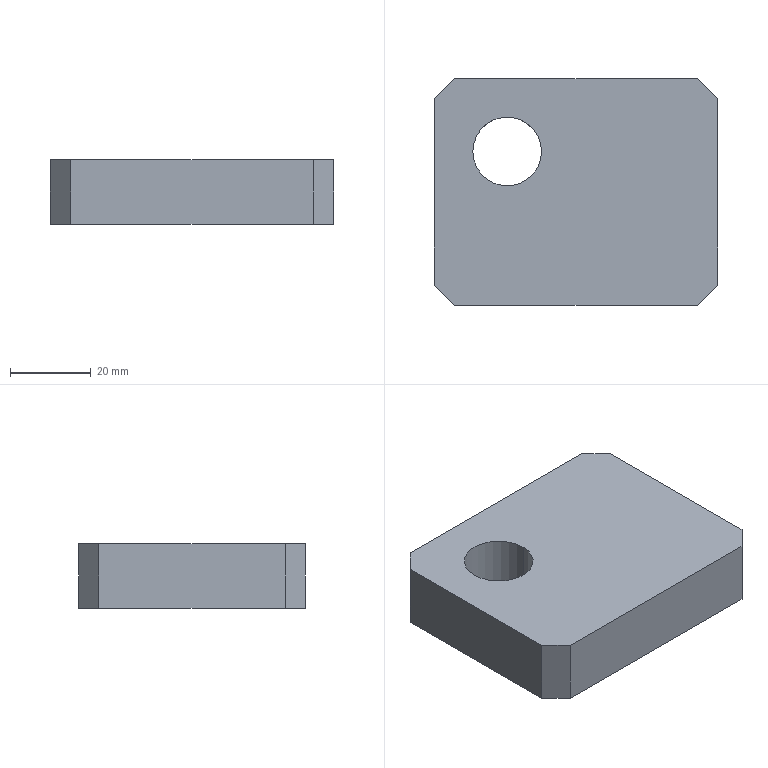Part | SolidWorks | features FlatPattern 1, SMBaseFlange 1, SheetMetal 1 | 1 solid | 12 faces | box 70 x 56 x 16 mm | volume 58288 mm3 | plane 10 | cylinder 2 | commonest cylinder face diameters 17 x2
STEP:
#1=CARTESIAN_POINT('',(9.5,-18.,-16.));
#2=VERTEX_POINT('',#1);
#3=CARTESIAN_POINT('',(26.5,-18.,-16.));
#4=VERTEX_POINT('',#3);
#5=CARTESIAN_POINT('',(18.,-18.,-16.));
#6=DIRECTION('',(0.,0.,1.));
#7=DIRECTION('',(1.,0.,0.));
#8=AXIS2_PLACEMENT_3D('',#5,#6,#7);
#9=CIRCLE('',#8,8.5);
#10=EDGE_CURVE('',#2,#4,#9,.T.);
#11=ORIENTED_EDGE('',*,*,#10,.F.);
#12=CARTESIAN_POINT('',(9.5,-18.,0.));
#13=VERTEX_POINT('',#12);
#14=CARTESIAN_POINT('',(9.5,-18.,-16.));
#15=DIRECTION('',(0.,0.,1.));
#16=VECTOR('',#15,1000.);
#17=LINE('',#14,#16);
#18=EDGE_CURVE('',#2,#13,#17,.T.);
#19=ORIENTED_EDGE('',*,*,#18,.T.);
#20=CARTESIAN_POINT('',(26.5,-18.,0.));
#21=VERTEX_POINT('',#20);
#22=CARTESIAN_POINT('',(18.,-18.,0.));
#23=DIRECTION('',(0.,0.,1.));
#24=DIRECTION('',(1.,0.,0.));
#25=AXIS2_PLACEMENT_3D('',#22,#23,#24);
#26=CIRCLE('',#25,8.5);
#27=EDGE_CURVE('',#13,#21,#26,.T.);
#28=ORIENTED_EDGE('',*,*,#27,.T.);
#29=CARTESIAN_POINT('',(26.5,-18.,-16.));
#30=DIRECTION('',(0.,0.,1.));
#31=VECTOR('',#30,1000.);
#32=LINE('',#29,#31);
#33=EDGE_CURVE('',#4,#21,#32,.T.);
#34=ORIENTED_EDGE('',*,*,#33,.F.);
#35=EDGE_LOOP('',(#11,#19,#28,#34));
#36=FACE_OUTER_BOUND('',#35,.T.);
#37=CARTESIAN_POINT('',(18.,-18.,-16.));
#38=DIRECTION('',(0.,0.,1.));
#39=DIRECTION('',(1.,0.,0.));
#40=AXIS2_PLACEMENT_3D('',#37,#38,#39);
#41=CYLINDRICAL_SURFACE('',#40,8.5);
#42=ADVANCED_FACE('',(#36),#41,.F.);
#43=CARTESIAN_POINT('',(65.,0.,0.));
#44=VERTEX_POINT('',#43);
#45=CARTESIAN_POINT('',(5.,0.,0.));
#46=VERTEX_POINT('',#45);
#47=CARTESIAN_POINT('',(5.,0.,0.));
#48=DIRECTION('',(-1.,0.,0.));
#49=VECTOR('',#48,1000.);
#50=LINE('',#47,#49);
#51=EDGE_CURVE('',#44,#46,#50,.T.);
#52=ORIENTED_EDGE('',*,*,#51,.F.);
#53=CARTESIAN_POINT('',(65.,0.,-16.));
#54=VERTEX_POINT('',#53);
#55=CARTESIAN_POINT('',(65.,0.,-16.));
#56=DIRECTION('',(0.,0.,1.));
#57=VECTOR('',#56,1000.);
#58=LINE('',#55,#57);
#59=EDGE_CURVE('',#54,#44,#58,.T.);
#60=ORIENTED_EDGE('',*,*,#59,.F.);
#61=CARTESIAN_POINT('',(5.,0.,-16.));
#62=VERTEX_POINT('',#61);
#63=CARTESIAN_POINT('',(5.,0.,-16.));
#64=DIRECTION('',(-1.,0.,0.));
#65=VECTOR('',#64,1000.);
#66=LINE('',#63,#65);
#67=EDGE_CURVE('',#54,#62,#66,.T.);
#68=ORIENTED_EDGE('',*,*,#67,.T.);
#69=CARTESIAN_POINT('',(5.,0.,-16.));
#70=DIRECTION('',(0.,0.,1.));
#71=VECTOR('',#70,1000.);
#72=LINE('',#69,#71);
#73=EDGE_CURVE('',#62,#46,#72,.T.);
#74=ORIENTED_EDGE('',*,*,#73,.T.);
#75=EDGE_LOOP('',(#52,#60,#68,#74));
#76=FACE_OUTER_BOUND('',#75,.T.);
#77=CARTESIAN_POINT('',(5.,0.,-16.));
#78=DIRECTION('',(0.,1.,0.));
#79=DIRECTION('',(0.,0.,1.));
#80=AXIS2_PLACEMENT_3D('',#77,#78,#79);
#81=PLANE('',#80);
#82=ADVANCED_FACE('',(#76),#81,.T.);
#83=CARTESIAN_POINT('',(70.,-5.,0.));
#84=VERTEX_POINT('',#83);
#85=CARTESIAN_POINT('',(65.,0.,0.));
#86=DIRECTION('',(-0.7071,0.7071,0.));
#87=VECTOR('',#86,1000.);
#88=LINE('',#85,#87);
#89=EDGE_CURVE('',#84,#44,#88,.T.);
#90=ORIENTED_EDGE('',*,*,#89,.F.);
#91=CARTESIAN_POINT('',(70.,-5.,-16.));
#92=VERTEX_POINT('',#91);
#93=CARTESIAN_POINT('',(70.,-5.,-16.));
#94=DIRECTION('',(0.,0.,1.));
#95=VECTOR('',#94,1000.);
#96=LINE('',#93,#95);
#97=EDGE_CURVE('',#92,#84,#96,.T.);
#98=ORIENTED_EDGE('',*,*,#97,.F.);
#99=CARTESIAN_POINT('',(65.,0.,-16.));
#100=DIRECTION('',(-0.7071,0.7071,0.));
#101=VECTOR('',#100,1000.);
#102=LINE('',#99,#101);
#103=EDGE_CURVE('',#92,#54,#102,.T.);
#104=ORIENTED_EDGE('',*,*,#103,.T.);
#105=ORIENTED_EDGE('',*,*,#59,.T.);
#106=EDGE_LOOP('',(#90,#98,#104,#105));
#107=FACE_OUTER_BOUND('',#106,.T.);
#108=CARTESIAN_POINT('',(65.,0.,-16.));
#109=DIRECTION('',(0.7071,0.7071,0.));
#110=DIRECTION('',(-0.7071,0.7071,0.));
#111=AXIS2_PLACEMENT_3D('',#108,#109,#110);
#112=PLANE('',#111);
#113=ADVANCED_FACE('',(#107),#112,.T.);
#114=CARTESIAN_POINT('',(70.,-51.,0.));
#115=VERTEX_POINT('',#114);
#116=CARTESIAN_POINT('',(70.,-5.,0.));
#117=DIRECTION('',(0.,1.,0.));
#118=VECTOR('',#117,1000.);
#119=LINE('',#116,#118);
#120=EDGE_CURVE('',#115,#84,#119,.T.);
#121=ORIENTED_EDGE('',*,*,#120,.F.);
#122=CARTESIAN_POINT('',(70.,-51.,-16.));
#123=VERTEX_POINT('',#122);
#124=CARTESIAN_POINT('',(70.,-51.,-16.));
#125=DIRECTION('',(0.,0.,1.));
#126=VECTOR('',#125,1000.);
#127=LINE('',#124,#126);
#128=EDGE_CURVE('',#123,#115,#127,.T.);
#129=ORIENTED_EDGE('',*,*,#128,.F.);
#130=CARTESIAN_POINT('',(70.,-5.,-16.));
#131=DIRECTION('',(0.,1.,0.));
#132=VECTOR('',#131,1000.);
#133=LINE('',#130,#132);
#134=EDGE_CURVE('',#123,#92,#133,.T.);
#135=ORIENTED_EDGE('',*,*,#134,.T.);
#136=ORIENTED_EDGE('',*,*,#97,.T.);
#137=EDGE_LOOP('',(#121,#129,#135,#136));
#138=FACE_OUTER_BOUND('',#137,.T.);
#139=CARTESIAN_POINT('',(70.,-5.,-16.));
#140=DIRECTION('',(1.,0.,0.));
#141=DIRECTION('',(0.,0.,-1.));
#142=AXIS2_PLACEMENT_3D('',#139,#140,#141);
#143=PLANE('',#142);
#144=ADVANCED_FACE('',(#138),#143,.T.);
#145=CARTESIAN_POINT('',(65.,-56.,0.));
#146=VERTEX_POINT('',#145);
#147=CARTESIAN_POINT('',(65.,-56.,0.));
#148=DIRECTION('',(0.7071,0.7071,0.));
#149=VECTOR('',#148,1000.);
#150=LINE('',#147,#149);
#151=EDGE_CURVE('',#146,#115,#150,.T.);
#152=ORIENTED_EDGE('',*,*,#151,.F.);
#153=CARTESIAN_POINT('',(65.,-56.,-16.));
#154=VERTEX_POINT('',#153);
#155=CARTESIAN_POINT('',(65.,-56.,-16.));
#156=DIRECTION('',(0.,0.,1.));
#157=VECTOR('',#156,1000.);
#158=LINE('',#155,#157);
#159=EDGE_CURVE('',#154,#146,#158,.T.);
#160=ORIENTED_EDGE('',*,*,#159,.F.);
#161=CARTESIAN_POINT('',(65.,-56.,-16.));
#162=DIRECTION('',(0.7071,0.7071,0.));
#163=VECTOR('',#162,1000.);
#164=LINE('',#161,#163);
#165=EDGE_CURVE('',#154,#123,#164,.T.);
#166=ORIENTED_EDGE('',*,*,#165,.T.);
#167=ORIENTED_EDGE('',*,*,#128,.T.);
#168=EDGE_LOOP('',(#152,#160,#166,#167));
#169=FACE_OUTER_BOUND('',#168,.T.);
#170=CARTESIAN_POINT('',(65.,-56.,-16.));
#171=DIRECTION('',(0.7071,-0.7071,0.));
#172=DIRECTION('',(0.7071,0.7071,0.));
#173=AXIS2_PLACEMENT_3D('',#170,#171,#172);
#174=PLANE('',#173);
#175=ADVANCED_FACE('',(#169),#174,.T.);
#176=CARTESIAN_POINT('',(5.,-56.,0.));
#177=VERTEX_POINT('',#176);
#178=CARTESIAN_POINT('',(5.,-56.,0.));
#179=DIRECTION('',(1.,0.,0.));
#180=VECTOR('',#179,1000.);
#181=LINE('',#178,#180);
#182=EDGE_CURVE('',#177,#146,#181,.T.);
#183=ORIENTED_EDGE('',*,*,#182,.F.);
#184=CARTESIAN_POINT('',(5.,-56.,-16.));
#185=VERTEX_POINT('',#184);
#186=CARTESIAN_POINT('',(5.,-56.,-16.));
#187=DIRECTION('',(0.,0.,1.));
#188=VECTOR('',#187,1000.);
#189=LINE('',#186,#188);
#190=EDGE_CURVE('',#185,#177,#189,.T.);
#191=ORIENTED_EDGE('',*,*,#190,.F.);
#192=CARTESIAN_POINT('',(5.,-56.,-16.));
#193=DIRECTION('',(1.,0.,0.));
#194=VECTOR('',#193,1000.);
#195=LINE('',#192,#194);
#196=EDGE_CURVE('',#185,#154,#195,.T.);
#197=ORIENTED_EDGE('',*,*,#196,.T.);
#198=ORIENTED_EDGE('',*,*,#159,.T.);
#199=EDGE_LOOP('',(#183,#191,#197,#198));
#200=FACE_OUTER_BOUND('',#199,.T.);
#201=CARTESIAN_POINT('',(5.,-56.,-16.));
#202=DIRECTION('',(0.,-1.,0.));
#203=DIRECTION('',(0.,0.,-1.));
#204=AXIS2_PLACEMENT_3D('',#201,#202,#203);
#205=PLANE('',#204);
#206=ADVANCED_FACE('',(#200),#205,.T.);
#207=CARTESIAN_POINT('',(0.,-51.,0.));
#208=VERTEX_POINT('',#207);
#209=CARTESIAN_POINT('',(0.,-51.,0.));
#210=DIRECTION('',(0.7071,-0.7071,0.));
#211=VECTOR('',#210,1000.);
#212=LINE('',#209,#211);
#213=EDGE_CURVE('',#208,#177,#212,.T.);
#214=ORIENTED_EDGE('',*,*,#213,.F.);
#215=CARTESIAN_POINT('',(0.,-51.,-16.));
#216=VERTEX_POINT('',#215);
#217=CARTESIAN_POINT('',(0.,-51.,-16.));
#218=DIRECTION('',(0.,0.,1.));
#219=VECTOR('',#218,1000.);
#220=LINE('',#217,#219);
#221=EDGE_CURVE('',#216,#208,#220,.T.);
#222=ORIENTED_EDGE('',*,*,#221,.F.);
#223=CARTESIAN_POINT('',(0.,-51.,-16.));
#224=DIRECTION('',(0.7071,-0.7071,0.));
#225=VECTOR('',#224,1000.);
#226=LINE('',#223,#225);
#227=EDGE_CURVE('',#216,#185,#226,.T.);
#228=ORIENTED_EDGE('',*,*,#227,.T.);
#229=ORIENTED_EDGE('',*,*,#190,.T.);
#230=EDGE_LOOP('',(#214,#222,#228,#229));
#231=FACE_OUTER_BOUND('',#230,.T.);
#232=CARTESIAN_POINT('',(0.,-51.,-16.));
#233=DIRECTION('',(-0.7071,-0.7071,0.));
#234=DIRECTION('',(0.7071,-0.7071,0.));
#235=AXIS2_PLACEMENT_3D('',#232,#233,#234);
#236=PLANE('',#235);
#237=ADVANCED_FACE('',(#231),#236,.T.);
#238=CARTESIAN_POINT('',(0.,-5.,0.));
#239=VERTEX_POINT('',#238);
#240=CARTESIAN_POINT('',(0.,-5.,0.));
#241=DIRECTION('',(0.,-1.,0.));
#242=VECTOR('',#241,1000.);
#243=LINE('',#240,#242);
#244=EDGE_CURVE('',#239,#208,#243,.T.);
#245=ORIENTED_EDGE('',*,*,#244,.F.);
#246=CARTESIAN_POINT('',(0.,-5.,-16.));
#247=VERTEX_POINT('',#246);
#248=CARTESIAN_POINT('',(0.,-5.,-16.));
#249=DIRECTION('',(0.,0.,1.));
#250=VECTOR('',#249,1000.);
#251=LINE('',#248,#250);
#252=EDGE_CURVE('',#247,#239,#251,.T.);
#253=ORIENTED_EDGE('',*,*,#252,.F.);
#254=CARTESIAN_POINT('',(0.,-5.,-16.));
#255=DIRECTION('',(0.,-1.,0.));
#256=VECTOR('',#255,1000.);
#257=LINE('',#254,#256);
#258=EDGE_CURVE('',#247,#216,#257,.T.);
#259=ORIENTED_EDGE('',*,*,#258,.T.);
#260=ORIENTED_EDGE('',*,*,#221,.T.);
#261=EDGE_LOOP('',(#245,#253,#259,#260));
#262=FACE_OUTER_BOUND('',#261,.T.);
#263=CARTESIAN_POINT('',(0.,-5.,-16.));
#264=DIRECTION('',(-1.,0.,0.));
#265=DIRECTION('',(0.,-1.,0.));
#266=AXIS2_PLACEMENT_3D('',#263,#264,#265);
#267=PLANE('',#266);
#268=ADVANCED_FACE('',(#262),#267,.T.);
#269=CARTESIAN_POINT('',(0.,-5.,0.));
#270=DIRECTION('',(-0.7071,-0.7071,0.));
#271=VECTOR('',#270,1000.);
#272=LINE('',#269,#271);
#273=EDGE_CURVE('',#46,#239,#272,.T.);
#274=ORIENTED_EDGE('',*,*,#273,.F.);
#275=ORIENTED_EDGE('',*,*,#73,.F.);
#276=CARTESIAN_POINT('',(0.,-5.,-16.));
#277=DIRECTION('',(-0.7071,-0.7071,0.));
#278=VECTOR('',#277,1000.);
#279=LINE('',#276,#278);
#280=EDGE_CURVE('',#62,#247,#279,.T.);
#281=ORIENTED_EDGE('',*,*,#280,.T.);
#282=ORIENTED_EDGE('',*,*,#252,.T.);
#283=EDGE_LOOP('',(#274,#275,#281,#282));
#284=FACE_OUTER_BOUND('',#283,.T.);
#285=CARTESIAN_POINT('',(0.,-5.,-16.));
#286=DIRECTION('',(-0.7071,0.7071,0.));
#287=DIRECTION('',(-0.7071,-0.7071,0.));
#288=AXIS2_PLACEMENT_3D('',#285,#286,#287);
#289=PLANE('',#288);
#290=ADVANCED_FACE('',(#284),#289,.T.);
#291=CARTESIAN_POINT('',(18.,-18.,-16.));
#292=DIRECTION('',(0.,0.,1.));
#293=DIRECTION('',(1.,0.,0.));
#294=AXIS2_PLACEMENT_3D('',#291,#292,#293);
#295=CIRCLE('',#294,8.5);
#296=EDGE_CURVE('',#4,#2,#295,.T.);
#297=ORIENTED_EDGE('',*,*,#296,.T.);
#298=ORIENTED_EDGE('',*,*,#10,.T.);
#299=EDGE_LOOP('',(#297,#298));
#300=FACE_BOUND('',#299,.T.);
#301=ORIENTED_EDGE('',*,*,#67,.F.);
#302=ORIENTED_EDGE('',*,*,#103,.F.);
#303=ORIENTED_EDGE('',*,*,#134,.F.);
#304=ORIENTED_EDGE('',*,*,#165,.F.);
#305=ORIENTED_EDGE('',*,*,#196,.F.);
#306=ORIENTED_EDGE('',*,*,#227,.F.);
#307=ORIENTED_EDGE('',*,*,#258,.F.);
#308=ORIENTED_EDGE('',*,*,#280,.F.);
#309=EDGE_LOOP('',(#301,#302,#303,#304,#305,#306,#307,#308));
#310=FACE_OUTER_BOUND('',#309,.T.);
#311=CARTESIAN_POINT('',(0.,0.,-16.));
#312=DIRECTION('',(0.,0.,-1.));
#313=DIRECTION('',(-1.,0.,0.));
#314=AXIS2_PLACEMENT_3D('',#311,#312,#313);
#315=PLANE('',#314);
#316=ADVANCED_FACE('',(#300,#310),#315,.T.);
#317=CARTESIAN_POINT('',(18.,-18.,0.));
#318=DIRECTION('',(0.,0.,1.));
#319=DIRECTION('',(1.,0.,0.));
#320=AXIS2_PLACEMENT_3D('',#317,#318,#319);
#321=CIRCLE('',#320,8.5);
#322=EDGE_CURVE('',#21,#13,#321,.T.);
#323=ORIENTED_EDGE('',*,*,#322,.F.);
#324=ORIENTED_EDGE('',*,*,#27,.F.);
#325=EDGE_LOOP('',(#323,#324));
#326=FACE_BOUND('',#325,.T.);
#327=ORIENTED_EDGE('',*,*,#51,.T.);
#328=ORIENTED_EDGE('',*,*,#273,.T.);
#329=ORIENTED_EDGE('',*,*,#244,.T.);
#330=ORIENTED_EDGE('',*,*,#213,.T.);
#331=ORIENTED_EDGE('',*,*,#182,.T.);
#332=ORIENTED_EDGE('',*,*,#151,.T.);
#333=ORIENTED_EDGE('',*,*,#120,.T.);
#334=ORIENTED_EDGE('',*,*,#89,.T.);
#335=EDGE_LOOP('',(#327,#328,#329,#330,#331,#332,#333,#334));
#336=FACE_OUTER_BOUND('',#335,.T.);
#337=CARTESIAN_POINT('',(0.,0.,0.));
#338=DIRECTION('',(0.,0.,-1.));
#339=DIRECTION('',(-1.,0.,0.));
#340=AXIS2_PLACEMENT_3D('',#337,#338,#339);
#341=PLANE('',#340);
#342=ADVANCED_FACE('',(#326,#336),#341,.F.);
#343=ORIENTED_EDGE('',*,*,#18,.F.);
#344=ORIENTED_EDGE('',*,*,#296,.F.);
#345=ORIENTED_EDGE('',*,*,#33,.T.);
#346=ORIENTED_EDGE('',*,*,#322,.T.);
#347=EDGE_LOOP('',(#343,#344,#345,#346));
#348=FACE_OUTER_BOUND('',#347,.T.);
#349=CARTESIAN_POINT('',(18.,-18.,-16.));
#350=DIRECTION('',(0.,0.,1.));
#351=DIRECTION('',(1.,0.,0.));
#352=AXIS2_PLACEMENT_3D('',#349,#350,#351);
#353=CYLINDRICAL_SURFACE('',#352,8.5);
#354=ADVANCED_FACE('',(#348),#353,.F.);
#355=CLOSED_SHELL('',(#42,#82,#113,#144,#175,#206,#237,#268,#290,#316,#342,#354));
#356=MANIFOLD_SOLID_BREP('',#355);
#357=CARTESIAN_POINT('',(0.,0.,0.));
#358=DIRECTION('',(0.,0.,1.));
#359=DIRECTION('',(1.,0.,0.));
#360=AXIS2_PLACEMENT_3D('',#357,#358,#359);
#361=(LENGTH_UNIT()NAMED_UNIT(*)SI_UNIT(.MILLI.,.METRE.));
#362=UNCERTAINTY_MEASURE_WITH_UNIT(LENGTH_MEASURE(0.00001),#361,'','');
#363=(NAMED_UNIT(*)PLANE_ANGLE_UNIT()SI_UNIT($,.RADIAN.));
#364=(NAMED_UNIT(*)SI_UNIT($,.STERADIAN.)SOLID_ANGLE_UNIT());
#365=(GEOMETRIC_REPRESENTATION_CONTEXT(3)GLOBAL_UNCERTAINTY_ASSIGNED_CONTEXT((#362))GLOBAL_UNIT_ASSIGNED_CONTEXT((#361,#363,#364))REPRESENTATION_CONTEXT('',''));
#366=ADVANCED_BREP_SHAPE_REPRESENTATION('',(#356,#360),#365);